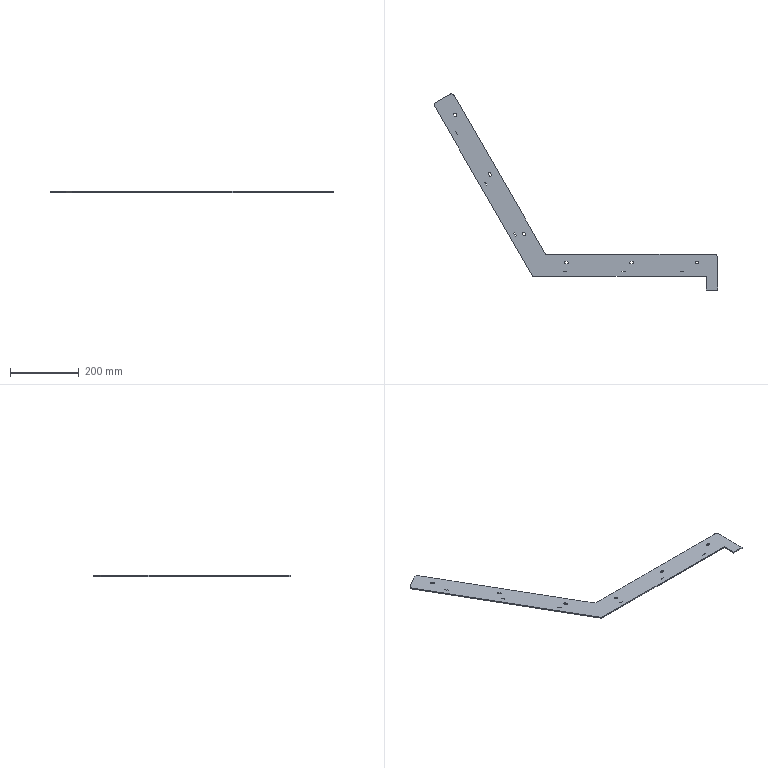Part | STEP file | zh004-2 | 1 solid | 67 faces | box 823.438 x 570.114 x 3 mm | volume 212618 mm3 | plane 46 | cylinder 21 | commonest cylinder face diameters 7 x18 20 x3